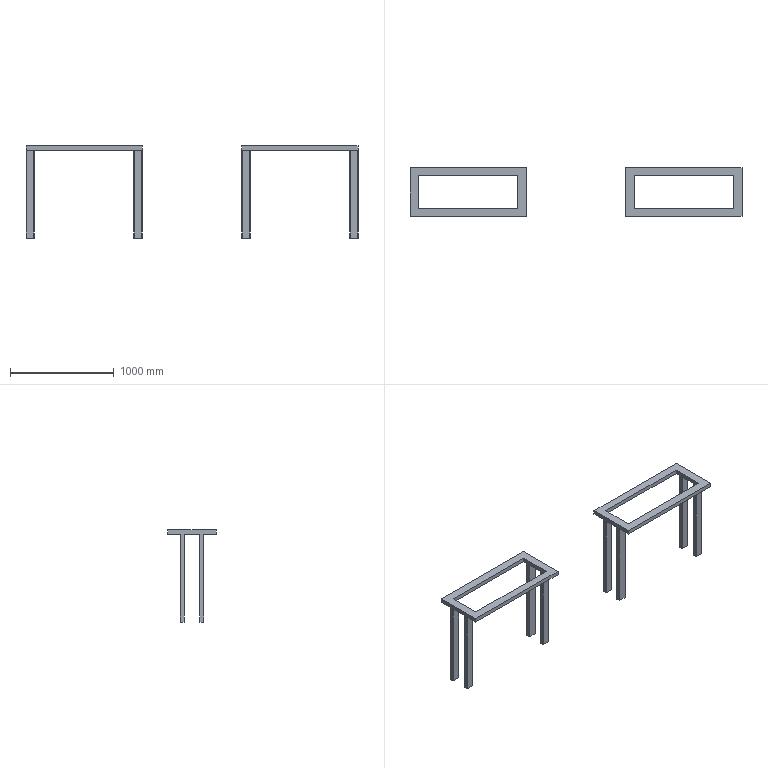Part | STEP file | Lower frame | 2 solids | 82 faces | box 3200 x 469.62 x 888 mm | volume 39914761 mm3 | plane 50 | cylinder 32 | commonest cylinder face diameters 8 x32